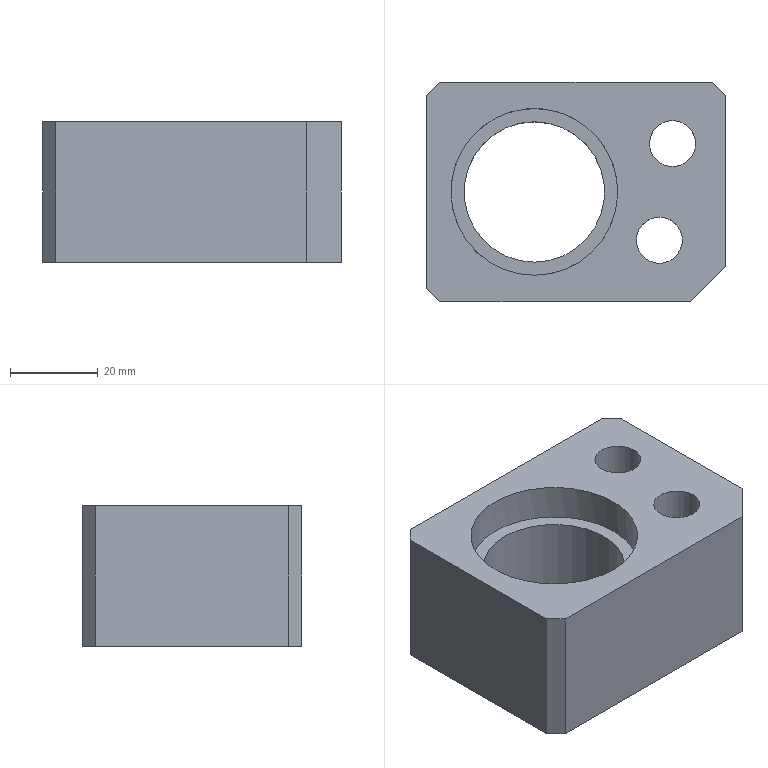Part | STEP file | lll_id3582_x_t | 1 solid | 19 faces | box 68 x 50 x 32 mm | volume 68588 mm3 | plane 13 | cylinder 6 | commonest cylinder face diameters 10.5 x2 17 x2 32 x1 38 x1
STEP:
#1=CARTESIAN_POINT('',(3228.727,-67.288,77.5));
#2=VERTEX_POINT('',#1);
#3=CARTESIAN_POINT('',(3233.977,-67.288,77.5));
#4=DIRECTION('',(0.,0.,1.));
#5=DIRECTION('',(-1.,0.,0.));
#6=AXIS2_PLACEMENT_3D('',#3,#4,#5);
#7=CIRCLE('',#6,5.25);
#8=EDGE_CURVE('',#2,#2,#7,.T.);
#9=ORIENTED_EDGE('',*,*,#8,.T.);
#10=EDGE_LOOP('',(#9));
#11=FACE_BOUND('',#10,.T.);
#12=CARTESIAN_POINT('',(3225.477,-67.288,77.5));
#13=VERTEX_POINT('',#12);
#14=CARTESIAN_POINT('',(3233.977,-67.288,77.5));
#15=DIRECTION('',(0.,0.,1.));
#16=DIRECTION('',(-1.,0.,0.));
#17=AXIS2_PLACEMENT_3D('',#14,#15,#16);
#18=CIRCLE('',#17,8.5);
#19=EDGE_CURVE('',#13,#13,#18,.T.);
#20=ORIENTED_EDGE('',*,*,#19,.F.);
#21=EDGE_LOOP('',(#20));
#22=FACE_BOUND('',#21,.T.);
#23=CARTESIAN_POINT('',(3233.977,-67.288,77.5));
#24=DIRECTION('',(0.,0.,1.));
#25=DIRECTION('',(0.,1.,0.));
#26=AXIS2_PLACEMENT_3D('',#23,#24,#25);
#27=PLANE('',#26);
#28=ADVANCED_FACE('',(#11,#22),#27,.F.);
#29=CARTESIAN_POINT('',(3205.477,-37.288,84.3));
#30=VERTEX_POINT('',#29);
#31=CARTESIAN_POINT('',(3205.477,-56.288,84.3));
#32=DIRECTION('',(0.,0.,1.));
#33=DIRECTION('',(0.,1.,0.));
#34=AXIS2_PLACEMENT_3D('',#31,#32,#33);
#35=CIRCLE('',#34,19.);
#36=EDGE_CURVE('',#30,#30,#35,.T.);
#37=ORIENTED_EDGE('',*,*,#36,.T.);
#38=EDGE_LOOP('',(#37));
#39=FACE_BOUND('',#38,.T.);
#40=CARTESIAN_POINT('',(3205.477,-40.288,84.3));
#41=VERTEX_POINT('',#40);
#42=CARTESIAN_POINT('',(3205.477,-56.288,84.3));
#43=DIRECTION('',(0.,0.,1.));
#44=DIRECTION('',(0.,1.,0.));
#45=AXIS2_PLACEMENT_3D('',#42,#43,#44);
#46=CIRCLE('',#45,16.);
#47=EDGE_CURVE('',#41,#41,#46,.T.);
#48=ORIENTED_EDGE('',*,*,#47,.F.);
#49=EDGE_LOOP('',(#48));
#50=FACE_BOUND('',#49,.T.);
#51=CARTESIAN_POINT('',(3214.227,-56.288,84.3));
#52=DIRECTION('',(0.,0.,-1.));
#53=DIRECTION('',(1.,0.,0.));
#54=AXIS2_PLACEMENT_3D('',#51,#52,#53);
#55=PLANE('',#54);
#56=ADVANCED_FACE('',(#39,#50),#55,.F.);
#57=ORIENTED_EDGE('',*,*,#19,.T.);
#58=EDGE_LOOP('',(#57));
#59=FACE_BOUND('',#58,.T.);
#60=CARTESIAN_POINT('',(3225.477,-67.288,60.5));
#61=VERTEX_POINT('',#60);
#62=CARTESIAN_POINT('',(3233.977,-67.288,60.5));
#63=DIRECTION('',(0.,0.,-1.));
#64=DIRECTION('',(-1.,0.,0.));
#65=AXIS2_PLACEMENT_3D('',#62,#63,#64);
#66=CIRCLE('',#65,8.5);
#67=EDGE_CURVE('',#61,#61,#66,.T.);
#68=ORIENTED_EDGE('',*,*,#67,.T.);
#69=EDGE_LOOP('',(#68));
#70=FACE_BOUND('',#69,.T.);
#71=CARTESIAN_POINT('',(3233.977,-67.288,60.5));
#72=DIRECTION('',(0.,0.,1.));
#73=DIRECTION('',(0.,1.,0.));
#74=AXIS2_PLACEMENT_3D('',#71,#72,#73);
#75=CYLINDRICAL_SURFACE('',#74,8.5);
#76=ADVANCED_FACE('',(#59,#70),#75,.F.);
#77=CARTESIAN_POINT('',(3183.977,-81.287,60.5));
#78=VERTEX_POINT('',#77);
#79=CARTESIAN_POINT('',(3180.977,-78.287,60.5));
#80=VERTEX_POINT('',#79);
#81=CARTESIAN_POINT('',(3164.794,-62.105,60.5));
#82=DIRECTION('',(-0.7071,0.7071,0.));
#83=VECTOR('',#82,1.);
#84=LINE('',#81,#83);
#85=EDGE_CURVE('',#78,#80,#84,.T.);
#86=ORIENTED_EDGE('',*,*,#85,.F.);
#87=CARTESIAN_POINT('',(3183.977,-81.287,92.5));
#88=VERTEX_POINT('',#87);
#89=CARTESIAN_POINT('',(3183.977,-81.287,-8.5));
#90=DIRECTION('',(0.,0.,-1.));
#91=VECTOR('',#90,1.);
#92=LINE('',#89,#91);
#93=EDGE_CURVE('',#88,#78,#92,.T.);
#94=ORIENTED_EDGE('',*,*,#93,.F.);
#95=CARTESIAN_POINT('',(3180.977,-78.287,92.5));
#96=VERTEX_POINT('',#95);
#97=CARTESIAN_POINT('',(3164.794,-62.105,92.5));
#98=DIRECTION('',(0.7071,-0.7071,0.));
#99=VECTOR('',#98,1.);
#100=LINE('',#97,#99);
#101=EDGE_CURVE('',#96,#88,#100,.T.);
#102=ORIENTED_EDGE('',*,*,#101,.F.);
#103=CARTESIAN_POINT('',(3180.977,-78.287,-8.5));
#104=DIRECTION('',(0.,0.,1.));
#105=VECTOR('',#104,1.);
#106=LINE('',#103,#105);
#107=EDGE_CURVE('',#80,#96,#106,.T.);
#108=ORIENTED_EDGE('',*,*,#107,.F.);
#109=EDGE_LOOP('',(#86,#94,#102,#108));
#110=FACE_OUTER_BOUND('',#109,.T.);
#111=CARTESIAN_POINT('',(3180.977,-78.287,-8.5));
#112=DIRECTION('',(0.7071,0.7071,0.));
#113=DIRECTION('',(0.,0.,1.));
#114=AXIS2_PLACEMENT_3D('',#111,#112,#113);
#115=PLANE('',#114);
#116=ADVANCED_FACE('',(#110),#115,.F.);
#117=CARTESIAN_POINT('',(3180.977,-34.288,60.5));
#118=VERTEX_POINT('',#117);
#119=CARTESIAN_POINT('',(3180.977,6.903,60.5));
#120=DIRECTION('',(0.,1.,0.));
#121=VECTOR('',#120,1.);
#122=LINE('',#119,#121);
#123=EDGE_CURVE('',#80,#118,#122,.T.);
#124=ORIENTED_EDGE('',*,*,#123,.F.);
#125=ORIENTED_EDGE('',*,*,#107,.T.);
#126=CARTESIAN_POINT('',(3180.977,-34.288,92.5));
#127=VERTEX_POINT('',#126);
#128=CARTESIAN_POINT('',(3180.977,-56.288,92.5));
#129=DIRECTION('',(0.,-1.,0.));
#130=VECTOR('',#129,1.);
#131=LINE('',#128,#130);
#132=EDGE_CURVE('',#127,#96,#131,.T.);
#133=ORIENTED_EDGE('',*,*,#132,.F.);
#134=CARTESIAN_POINT('',(3180.977,-34.288,-8.5));
#135=DIRECTION('',(0.,0.,1.));
#136=VECTOR('',#135,1.);
#137=LINE('',#134,#136);
#138=EDGE_CURVE('',#118,#127,#137,.T.);
#139=ORIENTED_EDGE('',*,*,#138,.F.);
#140=EDGE_LOOP('',(#124,#125,#133,#139));
#141=FACE_OUTER_BOUND('',#140,.T.);
#142=CARTESIAN_POINT('',(3180.977,-56.288,-8.5));
#143=DIRECTION('',(-1.,0.,0.));
#144=DIRECTION('',(0.,0.,-1.));
#145=AXIS2_PLACEMENT_3D('',#142,#143,#144);
#146=PLANE('',#145);
#147=ADVANCED_FACE('',(#141),#146,.T.);
#148=CARTESIAN_POINT('',(3183.977,-31.288,92.5));
#149=VERTEX_POINT('',#148);
#150=CARTESIAN_POINT('',(3183.977,-31.288,92.5));
#151=DIRECTION('',(0.7071,0.7071,0.));
#152=VECTOR('',#151,1.);
#153=LINE('',#150,#152);
#154=EDGE_CURVE('',#127,#149,#153,.T.);
#155=ORIENTED_EDGE('',*,*,#154,.T.);
#156=CARTESIAN_POINT('',(3183.977,-31.288,60.5));
#157=VERTEX_POINT('',#156);
#158=CARTESIAN_POINT('',(3183.977,-31.288,-8.5));
#159=DIRECTION('',(0.,0.,-1.));
#160=VECTOR('',#159,1.);
#161=LINE('',#158,#160);
#162=EDGE_CURVE('',#149,#157,#161,.T.);
#163=ORIENTED_EDGE('',*,*,#162,.T.);
#164=CARTESIAN_POINT('',(3179.027,-36.237,60.5));
#165=DIRECTION('',(-0.7071,-0.7071,0.));
#166=VECTOR('',#165,1.);
#167=LINE('',#164,#166);
#168=EDGE_CURVE('',#157,#118,#167,.T.);
#169=ORIENTED_EDGE('',*,*,#168,.T.);
#170=ORIENTED_EDGE('',*,*,#138,.T.);
#171=EDGE_LOOP('',(#155,#163,#169,#170));
#172=FACE_OUTER_BOUND('',#171,.T.);
#173=CARTESIAN_POINT('',(3183.977,-31.288,-8.5));
#174=DIRECTION('',(0.7071,-0.7071,0.));
#175=DIRECTION('',(0.7071,0.7071,0.));
#176=AXIS2_PLACEMENT_3D('',#173,#174,#175);
#177=PLANE('',#176);
#178=ADVANCED_FACE('',(#172),#177,.F.);
#179=CARTESIAN_POINT('',(3245.977,-31.288,60.5));
#180=VERTEX_POINT('',#179);
#181=CARTESIAN_POINT('',(3231.752,-31.288,60.5));
#182=DIRECTION('',(1.,0.,0.));
#183=VECTOR('',#182,1.);
#184=LINE('',#181,#183);
#185=EDGE_CURVE('',#157,#180,#184,.T.);
#186=ORIENTED_EDGE('',*,*,#185,.F.);
#187=ORIENTED_EDGE('',*,*,#162,.F.);
#188=CARTESIAN_POINT('',(3245.977,-31.288,92.5));
#189=VERTEX_POINT('',#188);
#190=CARTESIAN_POINT('',(3236.702,-31.288,92.5));
#191=DIRECTION('',(-1.,0.,0.));
#192=VECTOR('',#191,1.);
#193=LINE('',#190,#192);
#194=EDGE_CURVE('',#189,#149,#193,.T.);
#195=ORIENTED_EDGE('',*,*,#194,.F.);
#196=CARTESIAN_POINT('',(3245.977,-31.288,-8.5));
#197=DIRECTION('',(0.,0.,1.));
#198=VECTOR('',#197,1.);
#199=LINE('',#196,#198);
#200=EDGE_CURVE('',#180,#189,#199,.T.);
#201=ORIENTED_EDGE('',*,*,#200,.F.);
#202=EDGE_LOOP('',(#186,#187,#195,#201));
#203=FACE_OUTER_BOUND('',#202,.T.);
#204=CARTESIAN_POINT('',(3205.477,-31.288,-8.5));
#205=DIRECTION('',(0.,1.,0.));
#206=DIRECTION('',(0.,0.,-1.));
#207=AXIS2_PLACEMENT_3D('',#204,#205,#206);
#208=PLANE('',#207);
#209=ADVANCED_FACE('',(#203),#208,.T.);
#210=CARTESIAN_POINT('',(3248.977,-34.288,92.5));
#211=VERTEX_POINT('',#210);
#212=CARTESIAN_POINT('',(3248.977,-34.288,92.5));
#213=DIRECTION('',(0.7071,-0.7071,0.));
#214=VECTOR('',#213,1.);
#215=LINE('',#212,#214);
#216=EDGE_CURVE('',#189,#211,#215,.T.);
#217=ORIENTED_EDGE('',*,*,#216,.T.);
#218=CARTESIAN_POINT('',(3248.977,-34.288,60.5));
#219=VERTEX_POINT('',#218);
#220=CARTESIAN_POINT('',(3248.977,-34.288,-8.5));
#221=DIRECTION('',(0.,0.,-1.));
#222=VECTOR('',#221,1.);
#223=LINE('',#220,#222);
#224=EDGE_CURVE('',#211,#219,#223,.T.);
#225=ORIENTED_EDGE('',*,*,#224,.T.);
#226=CARTESIAN_POINT('',(3248.977,-34.288,60.5));
#227=DIRECTION('',(-0.7071,0.7071,0.));
#228=VECTOR('',#227,1.);
#229=LINE('',#226,#228);
#230=EDGE_CURVE('',#219,#180,#229,.T.);
#231=ORIENTED_EDGE('',*,*,#230,.T.);
#232=ORIENTED_EDGE('',*,*,#200,.T.);
#233=EDGE_LOOP('',(#217,#225,#231,#232));
#234=FACE_OUTER_BOUND('',#233,.T.);
#235=CARTESIAN_POINT('',(3248.977,-34.288,-8.5));
#236=DIRECTION('',(-0.7071,-0.7071,0.));
#237=DIRECTION('',(0.7071,-0.7071,0.));
#238=AXIS2_PLACEMENT_3D('',#235,#236,#237);
#239=PLANE('',#238);
#240=ADVANCED_FACE('',(#234),#239,.F.);
#241=CARTESIAN_POINT('',(3248.977,-73.287,92.5));
#242=VERTEX_POINT('',#241);
#243=CARTESIAN_POINT('',(3248.977,-56.288,92.5));
#244=DIRECTION('',(0.,1.,0.));
#245=VECTOR('',#244,1.);
#246=LINE('',#243,#245);
#247=EDGE_CURVE('',#242,#211,#246,.T.);
#248=ORIENTED_EDGE('',*,*,#247,.F.);
#249=CARTESIAN_POINT('',(3248.977,-73.287,60.5));
#250=VERTEX_POINT('',#249);
#251=CARTESIAN_POINT('',(3248.977,-73.287,-8.5));
#252=DIRECTION('',(0.,0.,-1.));
#253=VECTOR('',#252,1.);
#254=LINE('',#251,#253);
#255=EDGE_CURVE('',#242,#250,#254,.T.);
#256=ORIENTED_EDGE('',*,*,#255,.T.);
#257=CARTESIAN_POINT('',(3248.977,6.903,60.5));
#258=DIRECTION('',(0.,-1.,0.));
#259=VECTOR('',#258,1.);
#260=LINE('',#257,#259);
#261=EDGE_CURVE('',#219,#250,#260,.T.);
#262=ORIENTED_EDGE('',*,*,#261,.F.);
#263=ORIENTED_EDGE('',*,*,#224,.F.);
#264=EDGE_LOOP('',(#248,#256,#262,#263));
#265=FACE_OUTER_BOUND('',#264,.T.);
#266=CARTESIAN_POINT('',(3248.977,-56.288,-8.5));
#267=DIRECTION('',(1.,0.,0.));
#268=DIRECTION('',(0.,0.,1.));
#269=AXIS2_PLACEMENT_3D('',#266,#267,#268);
#270=PLANE('',#269);
#271=ADVANCED_FACE('',(#265),#270,.T.);
#272=CARTESIAN_POINT('',(3240.977,-81.287,92.5));
#273=VERTEX_POINT('',#272);
#274=CARTESIAN_POINT('',(3284.384,-37.88,92.5));
#275=DIRECTION('',(0.7071,0.7071,0.));
#276=VECTOR('',#275,1.);
#277=LINE('',#274,#276);
#278=EDGE_CURVE('',#273,#242,#277,.T.);
#279=ORIENTED_EDGE('',*,*,#278,.F.);
#280=CARTESIAN_POINT('',(3240.977,-81.287,60.5));
#281=VERTEX_POINT('',#280);
#282=CARTESIAN_POINT('',(3240.977,-81.287,-8.5));
#283=DIRECTION('',(0.,0.,1.));
#284=VECTOR('',#283,1.);
#285=LINE('',#282,#284);
#286=EDGE_CURVE('',#281,#273,#285,.T.);
#287=ORIENTED_EDGE('',*,*,#286,.F.);
#288=CARTESIAN_POINT('',(3279.434,-42.829,60.5));
#289=DIRECTION('',(-0.7071,-0.7071,0.));
#290=VECTOR('',#289,1.);
#291=LINE('',#288,#290);
#292=EDGE_CURVE('',#250,#281,#291,.T.);
#293=ORIENTED_EDGE('',*,*,#292,.F.);
#294=ORIENTED_EDGE('',*,*,#255,.F.);
#295=EDGE_LOOP('',(#279,#287,#293,#294));
#296=FACE_OUTER_BOUND('',#295,.T.);
#297=CARTESIAN_POINT('',(3248.977,-73.287,-8.5));
#298=DIRECTION('',(-0.7071,0.7071,0.));
#299=DIRECTION('',(0.,0.,-1.));
#300=AXIS2_PLACEMENT_3D('',#297,#298,#299);
#301=PLANE('',#300);
#302=ADVANCED_FACE('',(#296),#301,.F.);
#303=CARTESIAN_POINT('',(3231.752,-81.287,60.5));
#304=DIRECTION('',(-1.,0.,0.));
#305=VECTOR('',#304,1.);
#306=LINE('',#303,#305);
#307=EDGE_CURVE('',#281,#78,#306,.T.);
#308=ORIENTED_EDGE('',*,*,#307,.F.);
#309=ORIENTED_EDGE('',*,*,#286,.T.);
#310=CARTESIAN_POINT('',(3231.752,-81.287,92.5));
#311=DIRECTION('',(1.,0.,0.));
#312=VECTOR('',#311,1.);
#313=LINE('',#310,#312);
#314=EDGE_CURVE('',#88,#273,#313,.T.);
#315=ORIENTED_EDGE('',*,*,#314,.F.);
#316=ORIENTED_EDGE('',*,*,#93,.T.);
#317=EDGE_LOOP('',(#308,#309,#315,#316));
#318=FACE_OUTER_BOUND('',#317,.T.);
#319=CARTESIAN_POINT('',(3200.527,-81.287,-8.5));
#320=DIRECTION('',(0.,-1.,0.));
#321=DIRECTION('',(0.,0.,1.));
#322=AXIS2_PLACEMENT_3D('',#319,#320,#321);
#323=PLANE('',#322);
#324=ADVANCED_FACE('',(#318),#323,.T.);
#325=CARTESIAN_POINT('',(3228.727,-67.288,92.5));
#326=VERTEX_POINT('',#325);
#327=CARTESIAN_POINT('',(3233.977,-67.288,92.5));
#328=DIRECTION('',(0.,0.,-1.));
#329=DIRECTION('',(-1.,0.,0.));
#330=AXIS2_PLACEMENT_3D('',#327,#328,#329);
#331=CIRCLE('',#330,5.25);
#332=EDGE_CURVE('',#326,#326,#331,.T.);
#333=ORIENTED_EDGE('',*,*,#332,.F.);
#334=EDGE_LOOP('',(#333));
#335=FACE_BOUND('',#334,.T.);
#336=ORIENTED_EDGE('',*,*,#8,.F.);
#337=EDGE_LOOP('',(#336));
#338=FACE_BOUND('',#337,.T.);
#339=CARTESIAN_POINT('',(3233.977,-67.288,160.5));
#340=DIRECTION('',(0.,0.,1.));
#341=DIRECTION('',(0.,1.,0.));
#342=AXIS2_PLACEMENT_3D('',#339,#340,#341);
#343=CYLINDRICAL_SURFACE('',#342,5.25);
#344=ADVANCED_FACE('',(#335,#338),#343,.F.);
#345=CARTESIAN_POINT('',(3205.477,-75.288,92.5));
#346=VERTEX_POINT('',#345);
#347=CARTESIAN_POINT('',(3205.477,-56.288,92.5));
#348=DIRECTION('',(0.,0.,-1.));
#349=DIRECTION('',(0.,-1.,0.));
#350=AXIS2_PLACEMENT_3D('',#347,#348,#349);
#351=CIRCLE('',#350,19.);
#352=EDGE_CURVE('',#346,#346,#351,.T.);
#353=ORIENTED_EDGE('',*,*,#352,.F.);
#354=EDGE_LOOP('',(#353));
#355=FACE_BOUND('',#354,.T.);
#356=ORIENTED_EDGE('',*,*,#36,.F.);
#357=EDGE_LOOP('',(#356));
#358=FACE_BOUND('',#357,.T.);
#359=CARTESIAN_POINT('',(3205.477,-56.288,90.));
#360=DIRECTION('',(0.,0.,-1.));
#361=DIRECTION('',(-1.,0.,0.));
#362=AXIS2_PLACEMENT_3D('',#359,#360,#361);
#363=CYLINDRICAL_SURFACE('',#362,19.);
#364=ADVANCED_FACE('',(#355,#358),#363,.F.);
#365=CARTESIAN_POINT('',(3242.227,-45.287,92.5));
#366=VERTEX_POINT('',#365);
#367=CARTESIAN_POINT('',(3236.977,-45.287,92.5));
#368=DIRECTION('',(0.,0.,1.));
#369=DIRECTION('',(1.,0.,0.));
#370=AXIS2_PLACEMENT_3D('',#367,#368,#369);
#371=CIRCLE('',#370,5.25);
#372=EDGE_CURVE('',#366,#366,#371,.T.);
#373=ORIENTED_EDGE('',*,*,#372,.F.);
#374=EDGE_LOOP('',(#373));
#375=FACE_BOUND('',#374,.T.);
#376=ORIENTED_EDGE('',*,*,#352,.T.);
#377=EDGE_LOOP('',(#376));
#378=FACE_BOUND('',#377,.T.);
#379=ORIENTED_EDGE('',*,*,#332,.T.);
#380=EDGE_LOOP('',(#379));
#381=FACE_BOUND('',#380,.T.);
#382=ORIENTED_EDGE('',*,*,#314,.T.);
#383=ORIENTED_EDGE('',*,*,#278,.T.);
#384=ORIENTED_EDGE('',*,*,#247,.T.);
#385=ORIENTED_EDGE('',*,*,#216,.F.);
#386=ORIENTED_EDGE('',*,*,#194,.T.);
#387=ORIENTED_EDGE('',*,*,#154,.F.);
#388=ORIENTED_EDGE('',*,*,#132,.T.);
#389=ORIENTED_EDGE('',*,*,#101,.T.);
#390=EDGE_LOOP('',(#382,#383,#384,#385,#386,#387,#388,#389));
#391=FACE_BOUND('',#390,.T.);
#392=CARTESIAN_POINT('',(3236.702,11.853,92.5));
#393=DIRECTION('',(0.,0.,1.));
#394=DIRECTION('',(0.,1.,0.));
#395=AXIS2_PLACEMENT_3D('',#392,#393,#394);
#396=PLANE('',#395);
#397=ADVANCED_FACE('',(#375,#378,#381,#391),#396,.T.);
#398=CARTESIAN_POINT('',(3205.477,-72.288,60.5));
#399=VERTEX_POINT('',#398);
#400=CARTESIAN_POINT('',(3205.477,-56.288,60.5));
#401=DIRECTION('',(0.,0.,1.));
#402=DIRECTION('',(0.,-1.,0.));
#403=AXIS2_PLACEMENT_3D('',#400,#401,#402);
#404=CIRCLE('',#403,16.);
#405=EDGE_CURVE('',#399,#399,#404,.T.);
#406=ORIENTED_EDGE('',*,*,#405,.F.);
#407=EDGE_LOOP('',(#406));
#408=FACE_BOUND('',#407,.T.);
#409=ORIENTED_EDGE('',*,*,#47,.T.);
#410=EDGE_LOOP('',(#409));
#411=FACE_BOUND('',#410,.T.);
#412=CARTESIAN_POINT('',(3205.477,-56.288,44.8));
#413=DIRECTION('',(0.,0.,-1.));
#414=DIRECTION('',(-1.,0.,0.));
#415=AXIS2_PLACEMENT_3D('',#412,#413,#414);
#416=CYLINDRICAL_SURFACE('',#415,16.);
#417=ADVANCED_FACE('',(#408,#411),#416,.F.);
#418=CARTESIAN_POINT('',(3245.477,-45.287,60.5));
#419=VERTEX_POINT('',#418);
#420=CARTESIAN_POINT('',(3236.977,-45.287,60.5));
#421=DIRECTION('',(0.,0.,-1.));
#422=DIRECTION('',(1.,0.,0.));
#423=AXIS2_PLACEMENT_3D('',#420,#421,#422);
#424=CIRCLE('',#423,8.5);
#425=EDGE_CURVE('',#419,#419,#424,.T.);
#426=ORIENTED_EDGE('',*,*,#425,.F.);
#427=EDGE_LOOP('',(#426));
#428=FACE_BOUND('',#427,.T.);
#429=ORIENTED_EDGE('',*,*,#405,.T.);
#430=EDGE_LOOP('',(#429));
#431=FACE_BOUND('',#430,.T.);
#432=ORIENTED_EDGE('',*,*,#261,.T.);
#433=ORIENTED_EDGE('',*,*,#292,.T.);
#434=ORIENTED_EDGE('',*,*,#307,.T.);
#435=ORIENTED_EDGE('',*,*,#85,.T.);
#436=ORIENTED_EDGE('',*,*,#123,.T.);
#437=ORIENTED_EDGE('',*,*,#168,.F.);
#438=ORIENTED_EDGE('',*,*,#185,.T.);
#439=ORIENTED_EDGE('',*,*,#230,.F.);
#440=EDGE_LOOP('',(#432,#433,#434,#435,#436,#437,#438,#439));
#441=FACE_BOUND('',#440,.T.);
#442=ORIENTED_EDGE('',*,*,#67,.F.);
#443=EDGE_LOOP('',(#442));
#444=FACE_BOUND('',#443,.T.);
#445=CARTESIAN_POINT('',(3231.752,6.903,60.5));
#446=DIRECTION('',(0.,0.,1.));
#447=DIRECTION('',(0.,1.,0.));
#448=AXIS2_PLACEMENT_3D('',#445,#446,#447);
#449=PLANE('',#448);
#450=ADVANCED_FACE('',(#428,#431,#441,#444),#449,.F.);
#451=CARTESIAN_POINT('',(3231.727,-45.287,77.5));
#452=VERTEX_POINT('',#451);
#453=CARTESIAN_POINT('',(3236.977,-45.287,77.5));
#454=DIRECTION('',(0.,0.,1.));
#455=DIRECTION('',(-1.,0.,0.));
#456=AXIS2_PLACEMENT_3D('',#453,#454,#455);
#457=CIRCLE('',#456,5.25);
#458=EDGE_CURVE('',#452,#452,#457,.T.);
#459=ORIENTED_EDGE('',*,*,#458,.T.);
#460=EDGE_LOOP('',(#459));
#461=FACE_BOUND('',#460,.T.);
#462=CARTESIAN_POINT('',(3228.477,-45.287,77.5));
#463=VERTEX_POINT('',#462);
#464=CARTESIAN_POINT('',(3236.977,-45.287,77.5));
#465=DIRECTION('',(0.,0.,1.));
#466=DIRECTION('',(-1.,0.,0.));
#467=AXIS2_PLACEMENT_3D('',#464,#465,#466);
#468=CIRCLE('',#467,8.5);
#469=EDGE_CURVE('',#463,#463,#468,.T.);
#470=ORIENTED_EDGE('',*,*,#469,.F.);
#471=EDGE_LOOP('',(#470));
#472=FACE_BOUND('',#471,.T.);
#473=CARTESIAN_POINT('',(3236.977,-45.287,77.5));
#474=DIRECTION('',(0.,0.,1.));
#475=DIRECTION('',(0.,-1.,0.));
#476=AXIS2_PLACEMENT_3D('',#473,#474,#475);
#477=PLANE('',#476);
#478=ADVANCED_FACE('',(#461,#472),#477,.F.);
#479=ORIENTED_EDGE('',*,*,#372,.T.);
#480=EDGE_LOOP('',(#479));
#481=FACE_BOUND('',#480,.T.);
#482=ORIENTED_EDGE('',*,*,#458,.F.);
#483=EDGE_LOOP('',(#482));
#484=FACE_BOUND('',#483,.T.);
#485=CARTESIAN_POINT('',(3236.977,-45.287,160.5));
#486=DIRECTION('',(0.,0.,1.));
#487=DIRECTION('',(0.,-1.,0.));
#488=AXIS2_PLACEMENT_3D('',#485,#486,#487);
#489=CYLINDRICAL_SURFACE('',#488,5.25);
#490=ADVANCED_FACE('',(#481,#484),#489,.F.);
#491=ORIENTED_EDGE('',*,*,#469,.T.);
#492=EDGE_LOOP('',(#491));
#493=FACE_BOUND('',#492,.T.);
#494=ORIENTED_EDGE('',*,*,#425,.T.);
#495=EDGE_LOOP('',(#494));
#496=FACE_BOUND('',#495,.T.);
#497=CARTESIAN_POINT('',(3236.977,-45.287,60.5));
#498=DIRECTION('',(0.,0.,1.));
#499=DIRECTION('',(0.,-1.,0.));
#500=AXIS2_PLACEMENT_3D('',#497,#498,#499);
#501=CYLINDRICAL_SURFACE('',#500,8.5);
#502=ADVANCED_FACE('',(#493,#496),#501,.F.);
#503=CLOSED_SHELL('',(#28,#56,#76,#116,#147,#178,#209,#240,#271,#302,#324,#344,#364,#397,#417,#450,#478,#490,#502));
#504=MANIFOLD_SOLID_BREP('',#503);
#505=(LENGTH_UNIT()NAMED_UNIT(*)SI_UNIT(.MILLI.,.METRE.));
#506=UNCERTAINTY_MEASURE_WITH_UNIT(LENGTH_MEASURE(0.00002),#505,'','');
#507=(NAMED_UNIT(*)PLANE_ANGLE_UNIT()SI_UNIT($,.RADIAN.));
#508=PLANE_ANGLE_MEASURE_WITH_UNIT(PLANE_ANGLE_MEASURE(0.01745),#507);
#509=DIMENSIONAL_EXPONENTS(0.,0.,0.,0.,0.,0.,0.);
#510=(CONVERSION_BASED_UNIT('DEGREE',#508)NAMED_UNIT(#509)PLANE_ANGLE_UNIT());
#511=(NAMED_UNIT(*)SI_UNIT($,.STERADIAN.)SOLID_ANGLE_UNIT());
#512=(GEOMETRIC_REPRESENTATION_CONTEXT(3)GLOBAL_UNCERTAINTY_ASSIGNED_CONTEXT((#506))GLOBAL_UNIT_ASSIGNED_CONTEXT((#505,#510,#511))REPRESENTATION_CONTEXT('',''));
#513=ADVANCED_BREP_SHAPE_REPRESENTATION('',(#504),#512);